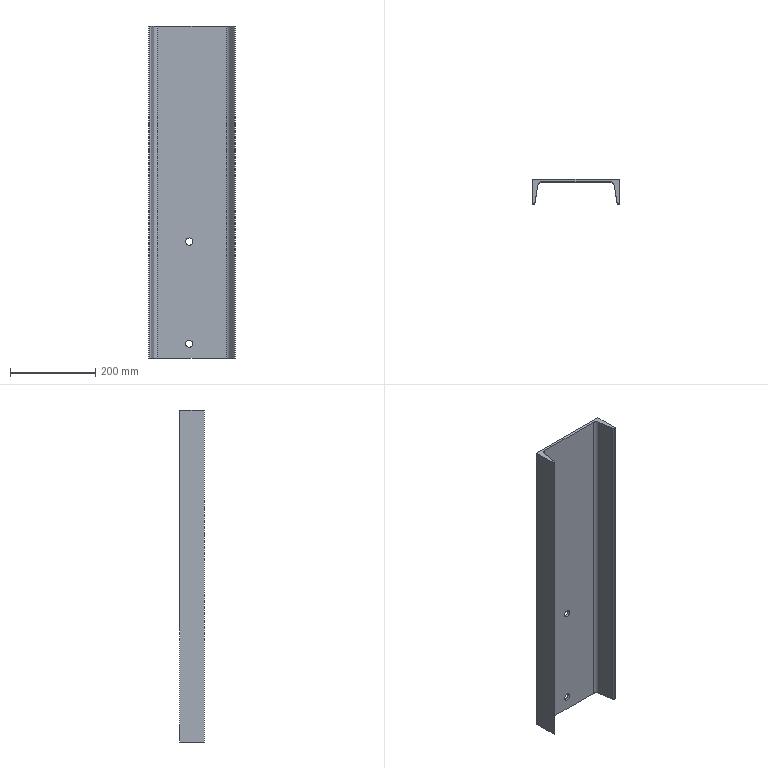Part | SolidWorks | features BaseBody 1 | 1 solid | 18 faces | box 203.2 x 57.4 x 780 mm | volume 1609191 mm3 | plane 10 | cylinder 8 | commonest cylinder face diameters 17 x4 6.6 x2 17.8 x2
STEP:
#1=CARTESIAN_POINT('',(61.02,28.984,265.));
#2=VERTEX_POINT('',#1);
#3=CARTESIAN_POINT('',(61.02,28.984,282.));
#4=VERTEX_POINT('',#3);
#5=CARTESIAN_POINT('',(61.02,28.984,273.5));
#6=DIRECTION('',(0.,1.,0.));
#7=DIRECTION('',(0.,0.,1.));
#8=AXIS2_PLACEMENT_3D('',#5,#6,#7);
#9=CIRCLE('',#8,8.5);
#10=EDGE_CURVE('',#2,#4,#9,.T.);
#11=ORIENTED_EDGE('',*,*,#10,.F.);
#12=CARTESIAN_POINT('',(61.02,34.584,265.));
#13=VERTEX_POINT('',#12);
#14=CARTESIAN_POINT('',(61.02,29.584,265.));
#15=DIRECTION('',(0.,1.,0.));
#16=VECTOR('',#15,1000.);
#17=LINE('',#14,#16);
#18=EDGE_CURVE('',#2,#13,#17,.T.);
#19=ORIENTED_EDGE('',*,*,#18,.T.);
#20=CARTESIAN_POINT('',(61.02,34.584,282.));
#21=VERTEX_POINT('',#20);
#22=CARTESIAN_POINT('',(61.02,34.584,273.5));
#23=DIRECTION('',(0.,-1.,0.));
#24=DIRECTION('',(0.,0.,1.));
#25=AXIS2_PLACEMENT_3D('',#22,#23,#24);
#26=CIRCLE('',#25,8.5);
#27=EDGE_CURVE('',#21,#13,#26,.T.);
#28=ORIENTED_EDGE('',*,*,#27,.F.);
#29=CARTESIAN_POINT('',(61.02,29.584,282.));
#30=DIRECTION('',(0.,1.,0.));
#31=VECTOR('',#30,1000.);
#32=LINE('',#29,#31);
#33=EDGE_CURVE('',#4,#21,#32,.T.);
#34=ORIENTED_EDGE('',*,*,#33,.F.);
#35=EDGE_LOOP('',(#11,#19,#28,#34));
#36=FACE_OUTER_BOUND('',#35,.T.);
#37=CARTESIAN_POINT('',(61.02,29.584,273.5));
#38=DIRECTION('',(0.,1.,0.));
#39=DIRECTION('',(0.,0.,1.));
#40=AXIS2_PLACEMENT_3D('',#37,#38,#39);
#41=CYLINDRICAL_SURFACE('',#40,8.5);
#42=ADVANCED_FACE('',(#36),#41,.F.);
#43=CARTESIAN_POINT('',(61.249,28.984,25.));
#44=VERTEX_POINT('',#43);
#45=CARTESIAN_POINT('',(61.249,28.984,42.));
#46=VERTEX_POINT('',#45);
#47=CARTESIAN_POINT('',(61.249,28.984,33.5));
#48=DIRECTION('',(0.,1.,0.));
#49=DIRECTION('',(0.,0.,1.));
#50=AXIS2_PLACEMENT_3D('',#47,#48,#49);
#51=CIRCLE('',#50,8.5);
#52=EDGE_CURVE('',#44,#46,#51,.T.);
#53=ORIENTED_EDGE('',*,*,#52,.F.);
#54=CARTESIAN_POINT('',(61.249,34.584,25.));
#55=VERTEX_POINT('',#54);
#56=CARTESIAN_POINT('',(61.249,29.584,25.));
#57=DIRECTION('',(0.,1.,0.));
#58=VECTOR('',#57,1000.);
#59=LINE('',#56,#58);
#60=EDGE_CURVE('',#44,#55,#59,.T.);
#61=ORIENTED_EDGE('',*,*,#60,.T.);
#62=CARTESIAN_POINT('',(61.249,34.584,42.));
#63=VERTEX_POINT('',#62);
#64=CARTESIAN_POINT('',(61.249,34.584,33.5));
#65=DIRECTION('',(0.,-1.,0.));
#66=DIRECTION('',(0.,0.,1.));
#67=AXIS2_PLACEMENT_3D('',#64,#65,#66);
#68=CIRCLE('',#67,8.5);
#69=EDGE_CURVE('',#63,#55,#68,.T.);
#70=ORIENTED_EDGE('',*,*,#69,.F.);
#71=CARTESIAN_POINT('',(61.249,29.584,42.));
#72=DIRECTION('',(0.,1.,0.));
#73=VECTOR('',#72,1000.);
#74=LINE('',#71,#73);
#75=EDGE_CURVE('',#46,#63,#74,.T.);
#76=ORIENTED_EDGE('',*,*,#75,.F.);
#77=EDGE_LOOP('',(#53,#61,#70,#76));
#78=FACE_OUTER_BOUND('',#77,.T.);
#79=CARTESIAN_POINT('',(61.249,29.584,33.5));
#80=DIRECTION('',(0.,1.,0.));
#81=DIRECTION('',(0.,0.,1.));
#82=AXIS2_PLACEMENT_3D('',#79,#80,#81);
#83=CYLINDRICAL_SURFACE('',#82,8.5);
#84=ADVANCED_FACE('',(#78),#83,.F.);
#85=ORIENTED_EDGE('',*,*,#27,.T.);
#86=CARTESIAN_POINT('',(61.02,34.584,273.5));
#87=DIRECTION('',(0.,-1.,0.));
#88=DIRECTION('',(0.,0.,1.));
#89=AXIS2_PLACEMENT_3D('',#86,#87,#88);
#90=CIRCLE('',#89,8.5);
#91=EDGE_CURVE('',#13,#21,#90,.T.);
#92=ORIENTED_EDGE('',*,*,#91,.T.);
#93=EDGE_LOOP('',(#85,#92));
#94=FACE_BOUND('',#93,.T.);
#95=ORIENTED_EDGE('',*,*,#69,.T.);
#96=CARTESIAN_POINT('',(61.249,34.584,33.5));
#97=DIRECTION('',(0.,-1.,0.));
#98=DIRECTION('',(0.,0.,1.));
#99=AXIS2_PLACEMENT_3D('',#96,#97,#98);
#100=CIRCLE('',#99,8.5);
#101=EDGE_CURVE('',#55,#63,#100,.T.);
#102=ORIENTED_EDGE('',*,*,#101,.T.);
#103=EDGE_LOOP('',(#95,#102));
#104=FACE_BOUND('',#103,.T.);
#105=CARTESIAN_POINT('',(169.22,34.584,0.));
#106=VERTEX_POINT('',#105);
#107=CARTESIAN_POINT('',(-33.98,34.584,0.));
#108=VERTEX_POINT('',#107);
#109=CARTESIAN_POINT('',(-33.98,34.584,0.));
#110=DIRECTION('',(-1.,0.,0.));
#111=VECTOR('',#110,1000.);
#112=LINE('',#109,#111);
#113=EDGE_CURVE('',#106,#108,#112,.T.);
#114=ORIENTED_EDGE('',*,*,#113,.T.);
#115=CARTESIAN_POINT('',(-33.98,34.584,780.));
#116=VERTEX_POINT('',#115);
#117=CARTESIAN_POINT('',(-33.98,34.584,0.));
#118=DIRECTION('',(0.,0.,1.));
#119=VECTOR('',#118,1000.);
#120=LINE('',#117,#119);
#121=EDGE_CURVE('',#108,#116,#120,.T.);
#122=ORIENTED_EDGE('',*,*,#121,.T.);
#123=CARTESIAN_POINT('',(169.22,34.584,780.));
#124=VERTEX_POINT('',#123);
#125=CARTESIAN_POINT('',(-33.98,34.584,780.));
#126=DIRECTION('',(1.,0.,0.));
#127=VECTOR('',#126,1000.);
#128=LINE('',#125,#127);
#129=EDGE_CURVE('',#116,#124,#128,.T.);
#130=ORIENTED_EDGE('',*,*,#129,.T.);
#131=CARTESIAN_POINT('',(169.22,34.584,0.));
#132=DIRECTION('',(0.,0.,-1.));
#133=VECTOR('',#132,1000.);
#134=LINE('',#131,#133);
#135=EDGE_CURVE('',#124,#106,#134,.T.);
#136=ORIENTED_EDGE('',*,*,#135,.T.);
#137=EDGE_LOOP('',(#114,#122,#130,#136));
#138=FACE_OUTER_BOUND('',#137,.T.);
#139=CARTESIAN_POINT('',(-33.98,34.584,0.));
#140=DIRECTION('',(0.,1.,0.));
#141=DIRECTION('',(0.,0.,1.));
#142=AXIS2_PLACEMENT_3D('',#139,#140,#141);
#143=PLANE('',#142);
#144=ADVANCED_FACE('',(#94,#104,#138),#143,.T.);
#145=ORIENTED_EDGE('',*,*,#18,.F.);
#146=CARTESIAN_POINT('',(61.02,28.984,273.5));
#147=DIRECTION('',(0.,1.,0.));
#148=DIRECTION('',(0.,0.,1.));
#149=AXIS2_PLACEMENT_3D('',#146,#147,#148);
#150=CIRCLE('',#149,8.5);
#151=EDGE_CURVE('',#4,#2,#150,.T.);
#152=ORIENTED_EDGE('',*,*,#151,.F.);
#153=ORIENTED_EDGE('',*,*,#33,.T.);
#154=ORIENTED_EDGE('',*,*,#91,.F.);
#155=EDGE_LOOP('',(#145,#152,#153,#154));
#156=FACE_OUTER_BOUND('',#155,.T.);
#157=CARTESIAN_POINT('',(61.02,29.584,273.5));
#158=DIRECTION('',(0.,1.,0.));
#159=DIRECTION('',(0.,0.,1.));
#160=AXIS2_PLACEMENT_3D('',#157,#158,#159);
#161=CYLINDRICAL_SURFACE('',#160,8.5);
#162=ADVANCED_FACE('',(#156),#161,.F.);
#163=ORIENTED_EDGE('',*,*,#60,.F.);
#164=CARTESIAN_POINT('',(61.249,28.984,33.5));
#165=DIRECTION('',(0.,1.,0.));
#166=DIRECTION('',(0.,0.,1.));
#167=AXIS2_PLACEMENT_3D('',#164,#165,#166);
#168=CIRCLE('',#167,8.5);
#169=EDGE_CURVE('',#46,#44,#168,.T.);
#170=ORIENTED_EDGE('',*,*,#169,.F.);
#171=ORIENTED_EDGE('',*,*,#75,.T.);
#172=ORIENTED_EDGE('',*,*,#101,.F.);
#173=EDGE_LOOP('',(#163,#170,#171,#172));
#174=FACE_OUTER_BOUND('',#173,.T.);
#175=CARTESIAN_POINT('',(61.249,29.584,33.5));
#176=DIRECTION('',(0.,1.,0.));
#177=DIRECTION('',(0.,0.,1.));
#178=AXIS2_PLACEMENT_3D('',#175,#176,#177);
#179=CYLINDRICAL_SURFACE('',#178,8.5);
#180=ADVANCED_FACE('',(#174),#179,.F.);
#181=CARTESIAN_POINT('',(-33.98,-22.816,0.));
#182=VERTEX_POINT('',#181);
#183=CARTESIAN_POINT('',(-33.98,-22.816,0.));
#184=DIRECTION('',(0.,-1.,0.));
#185=VECTOR('',#184,1000.);
#186=LINE('',#183,#185);
#187=EDGE_CURVE('',#108,#182,#186,.T.);
#188=ORIENTED_EDGE('',*,*,#187,.T.);
#189=CARTESIAN_POINT('',(-33.98,-22.816,780.));
#190=VERTEX_POINT('',#189);
#191=CARTESIAN_POINT('',(-33.98,-22.816,0.));
#192=DIRECTION('',(0.,0.,1.));
#193=VECTOR('',#192,1000.);
#194=LINE('',#191,#193);
#195=EDGE_CURVE('',#182,#190,#194,.T.);
#196=ORIENTED_EDGE('',*,*,#195,.T.);
#197=CARTESIAN_POINT('',(-33.98,-22.816,780.));
#198=DIRECTION('',(0.,1.,0.));
#199=VECTOR('',#198,1000.);
#200=LINE('',#197,#199);
#201=EDGE_CURVE('',#190,#116,#200,.T.);
#202=ORIENTED_EDGE('',*,*,#201,.T.);
#203=ORIENTED_EDGE('',*,*,#121,.F.);
#204=EDGE_LOOP('',(#188,#196,#202,#203));
#205=FACE_OUTER_BOUND('',#204,.T.);
#206=CARTESIAN_POINT('',(-33.98,-22.816,0.));
#207=DIRECTION('',(-1.,0.,0.));
#208=DIRECTION('',(0.,0.,1.));
#209=AXIS2_PLACEMENT_3D('',#206,#207,#208);
#210=PLANE('',#209);
#211=ADVANCED_FACE('',(#205),#210,.T.);
#212=CARTESIAN_POINT('',(167.576,-22.816,0.));
#213=VERTEX_POINT('',#212);
#214=CARTESIAN_POINT('',(169.22,-22.816,0.));
#215=VERTEX_POINT('',#214);
#216=CARTESIAN_POINT('',(169.22,-22.816,0.));
#217=DIRECTION('',(1.,0.,0.));
#218=VECTOR('',#217,1000.);
#219=LINE('',#216,#218);
#220=EDGE_CURVE('',#213,#215,#219,.T.);
#221=ORIENTED_EDGE('',*,*,#220,.F.);
#222=CARTESIAN_POINT('',(164.321,-20.06,0.));
#223=VERTEX_POINT('',#222);
#224=CARTESIAN_POINT('',(167.576,-19.516,0.));
#225=DIRECTION('',(0.,0.,1.));
#226=DIRECTION('',(1.,0.,0.));
#227=AXIS2_PLACEMENT_3D('',#224,#225,#226);
#228=CIRCLE('',#227,3.3);
#229=EDGE_CURVE('',#223,#213,#228,.T.);
#230=ORIENTED_EDGE('',*,*,#229,.F.);
#231=CARTESIAN_POINT('',(157.358,21.553,0.));
#232=VERTEX_POINT('',#231);
#233=CARTESIAN_POINT('',(157.358,21.553,0.));
#234=DIRECTION('',(0.165,-0.9863,0.));
#235=VECTOR('',#234,1000.);
#236=LINE('',#233,#235);
#237=EDGE_CURVE('',#232,#223,#236,.T.);
#238=ORIENTED_EDGE('',*,*,#237,.F.);
#239=CARTESIAN_POINT('',(148.58,28.984,0.));
#240=VERTEX_POINT('',#239);
#241=CARTESIAN_POINT('',(148.58,20.084,0.));
#242=DIRECTION('',(0.,0.,-1.));
#243=DIRECTION('',(1.,0.,0.));
#244=AXIS2_PLACEMENT_3D('',#241,#242,#243);
#245=CIRCLE('',#244,8.9);
#246=EDGE_CURVE('',#240,#232,#245,.T.);
#247=ORIENTED_EDGE('',*,*,#246,.F.);
#248=CARTESIAN_POINT('',(-13.34,28.984,0.));
#249=VERTEX_POINT('',#248);
#250=CARTESIAN_POINT('',(67.62,28.984,0.));
#251=DIRECTION('',(1.,0.,0.));
#252=VECTOR('',#251,1000.);
#253=LINE('',#250,#252);
#254=EDGE_CURVE('',#249,#240,#253,.T.);
#255=ORIENTED_EDGE('',*,*,#254,.F.);
#256=CARTESIAN_POINT('',(-22.118,21.553,0.));
#257=VERTEX_POINT('',#256);
#258=CARTESIAN_POINT('',(-13.34,20.084,0.));
#259=DIRECTION('',(0.,0.,-1.));
#260=DIRECTION('',(1.,0.,0.));
#261=AXIS2_PLACEMENT_3D('',#258,#259,#260);
#262=CIRCLE('',#261,8.9);
#263=EDGE_CURVE('',#257,#249,#262,.T.);
#264=ORIENTED_EDGE('',*,*,#263,.F.);
#265=CARTESIAN_POINT('',(-29.082,-20.06,0.));
#266=VERTEX_POINT('',#265);
#267=CARTESIAN_POINT('',(-29.082,-20.06,0.));
#268=DIRECTION('',(0.165,0.9863,0.));
#269=VECTOR('',#268,1000.);
#270=LINE('',#267,#269);
#271=EDGE_CURVE('',#266,#257,#270,.T.);
#272=ORIENTED_EDGE('',*,*,#271,.F.);
#273=CARTESIAN_POINT('',(-32.337,-22.816,0.));
#274=VERTEX_POINT('',#273);
#275=CARTESIAN_POINT('',(-32.337,-19.516,0.));
#276=DIRECTION('',(0.,0.,1.));
#277=DIRECTION('',(1.,0.,0.));
#278=AXIS2_PLACEMENT_3D('',#275,#276,#277);
#279=CIRCLE('',#278,3.3);
#280=EDGE_CURVE('',#274,#266,#279,.T.);
#281=ORIENTED_EDGE('',*,*,#280,.F.);
#282=CARTESIAN_POINT('',(67.62,-22.816,0.));
#283=DIRECTION('',(1.,0.,0.));
#284=VECTOR('',#283,1000.);
#285=LINE('',#282,#284);
#286=EDGE_CURVE('',#182,#274,#285,.T.);
#287=ORIENTED_EDGE('',*,*,#286,.F.);
#288=ORIENTED_EDGE('',*,*,#187,.F.);
#289=ORIENTED_EDGE('',*,*,#113,.F.);
#290=CARTESIAN_POINT('',(169.22,21.33,0.));
#291=DIRECTION('',(0.,1.,0.));
#292=VECTOR('',#291,1000.);
#293=LINE('',#290,#292);
#294=EDGE_CURVE('',#215,#106,#293,.T.);
#295=ORIENTED_EDGE('',*,*,#294,.F.);
#296=EDGE_LOOP('',(#221,#230,#238,#247,#255,#264,#272,#281,#287,#288,#289,#295));
#297=FACE_OUTER_BOUND('',#296,.T.);
#298=CARTESIAN_POINT('',(67.62,21.33,0.));
#299=DIRECTION('',(0.,0.,1.));
#300=DIRECTION('',(1.,0.,0.));
#301=AXIS2_PLACEMENT_3D('',#298,#299,#300);
#302=PLANE('',#301);
#303=ADVANCED_FACE('',(#297),#302,.F.);
#304=ORIENTED_EDGE('',*,*,#294,.T.);
#305=ORIENTED_EDGE('',*,*,#135,.F.);
#306=CARTESIAN_POINT('',(169.22,-22.816,780.));
#307=VERTEX_POINT('',#306);
#308=CARTESIAN_POINT('',(169.22,34.584,780.));
#309=DIRECTION('',(0.,-1.,0.));
#310=VECTOR('',#309,1000.);
#311=LINE('',#308,#310);
#312=EDGE_CURVE('',#124,#307,#311,.T.);
#313=ORIENTED_EDGE('',*,*,#312,.T.);
#314=CARTESIAN_POINT('',(169.22,-22.816,0.));
#315=DIRECTION('',(0.,0.,-1.));
#316=VECTOR('',#315,1000.);
#317=LINE('',#314,#316);
#318=EDGE_CURVE('',#307,#215,#317,.T.);
#319=ORIENTED_EDGE('',*,*,#318,.T.);
#320=EDGE_LOOP('',(#304,#305,#313,#319));
#321=FACE_OUTER_BOUND('',#320,.T.);
#322=CARTESIAN_POINT('',(169.22,34.584,0.));
#323=DIRECTION('',(1.,0.,0.));
#324=DIRECTION('',(0.,0.,-1.));
#325=AXIS2_PLACEMENT_3D('',#322,#323,#324);
#326=PLANE('',#325);
#327=ADVANCED_FACE('',(#321),#326,.T.);
#328=CARTESIAN_POINT('',(157.358,21.553,780.));
#329=VERTEX_POINT('',#328);
#330=CARTESIAN_POINT('',(164.321,-20.06,780.));
#331=VERTEX_POINT('',#330);
#332=CARTESIAN_POINT('',(157.358,21.553,780.));
#333=DIRECTION('',(0.165,-0.9863,0.));
#334=VECTOR('',#333,1000.);
#335=LINE('',#332,#334);
#336=EDGE_CURVE('',#329,#331,#335,.T.);
#337=ORIENTED_EDGE('',*,*,#336,.T.);
#338=CARTESIAN_POINT('',(167.576,-22.816,780.));
#339=VERTEX_POINT('',#338);
#340=CARTESIAN_POINT('',(167.576,-19.516,780.));
#341=DIRECTION('',(0.,0.,1.));
#342=DIRECTION('',(1.,0.,0.));
#343=AXIS2_PLACEMENT_3D('',#340,#341,#342);
#344=CIRCLE('',#343,3.3);
#345=EDGE_CURVE('',#331,#339,#344,.T.);
#346=ORIENTED_EDGE('',*,*,#345,.T.);
#347=CARTESIAN_POINT('',(67.62,-22.816,780.));
#348=DIRECTION('',(1.,0.,0.));
#349=VECTOR('',#348,1000.);
#350=LINE('',#347,#349);
#351=EDGE_CURVE('',#339,#307,#350,.T.);
#352=ORIENTED_EDGE('',*,*,#351,.T.);
#353=ORIENTED_EDGE('',*,*,#312,.F.);
#354=ORIENTED_EDGE('',*,*,#129,.F.);
#355=ORIENTED_EDGE('',*,*,#201,.F.);
#356=CARTESIAN_POINT('',(-32.337,-22.816,780.));
#357=VERTEX_POINT('',#356);
#358=CARTESIAN_POINT('',(67.62,-22.816,780.));
#359=DIRECTION('',(1.,0.,0.));
#360=VECTOR('',#359,1000.);
#361=LINE('',#358,#360);
#362=EDGE_CURVE('',#190,#357,#361,.T.);
#363=ORIENTED_EDGE('',*,*,#362,.T.);
#364=CARTESIAN_POINT('',(-29.082,-20.06,780.));
#365=VERTEX_POINT('',#364);
#366=CARTESIAN_POINT('',(-32.337,-19.516,780.));
#367=DIRECTION('',(0.,0.,1.));
#368=DIRECTION('',(1.,0.,0.));
#369=AXIS2_PLACEMENT_3D('',#366,#367,#368);
#370=CIRCLE('',#369,3.3);
#371=EDGE_CURVE('',#357,#365,#370,.T.);
#372=ORIENTED_EDGE('',*,*,#371,.T.);
#373=CARTESIAN_POINT('',(-22.118,21.553,780.));
#374=VERTEX_POINT('',#373);
#375=CARTESIAN_POINT('',(-29.082,-20.06,780.));
#376=DIRECTION('',(0.165,0.9863,0.));
#377=VECTOR('',#376,1000.);
#378=LINE('',#375,#377);
#379=EDGE_CURVE('',#365,#374,#378,.T.);
#380=ORIENTED_EDGE('',*,*,#379,.T.);
#381=CARTESIAN_POINT('',(-13.34,28.984,780.));
#382=VERTEX_POINT('',#381);
#383=CARTESIAN_POINT('',(-13.34,20.084,780.));
#384=DIRECTION('',(0.,0.,-1.));
#385=DIRECTION('',(1.,0.,0.));
#386=AXIS2_PLACEMENT_3D('',#383,#384,#385);
#387=CIRCLE('',#386,8.9);
#388=EDGE_CURVE('',#374,#382,#387,.T.);
#389=ORIENTED_EDGE('',*,*,#388,.T.);
#390=CARTESIAN_POINT('',(148.58,28.984,780.));
#391=VERTEX_POINT('',#390);
#392=CARTESIAN_POINT('',(67.62,28.984,780.));
#393=DIRECTION('',(1.,0.,0.));
#394=VECTOR('',#393,1000.);
#395=LINE('',#392,#394);
#396=EDGE_CURVE('',#382,#391,#395,.T.);
#397=ORIENTED_EDGE('',*,*,#396,.T.);
#398=CARTESIAN_POINT('',(148.58,20.084,780.));
#399=DIRECTION('',(0.,0.,-1.));
#400=DIRECTION('',(1.,0.,0.));
#401=AXIS2_PLACEMENT_3D('',#398,#399,#400);
#402=CIRCLE('',#401,8.9);
#403=EDGE_CURVE('',#391,#329,#402,.T.);
#404=ORIENTED_EDGE('',*,*,#403,.T.);
#405=EDGE_LOOP('',(#337,#346,#352,#353,#354,#355,#363,#372,#380,#389,#397,#404));
#406=FACE_OUTER_BOUND('',#405,.T.);
#407=CARTESIAN_POINT('',(67.62,21.33,780.));
#408=DIRECTION('',(0.,0.,1.));
#409=DIRECTION('',(1.,0.,0.));
#410=AXIS2_PLACEMENT_3D('',#407,#408,#409);
#411=PLANE('',#410);
#412=ADVANCED_FACE('',(#406),#411,.T.);
#413=ORIENTED_EDGE('',*,*,#151,.T.);
#414=ORIENTED_EDGE('',*,*,#10,.T.);
#415=EDGE_LOOP('',(#413,#414));
#416=FACE_BOUND('',#415,.T.);
#417=ORIENTED_EDGE('',*,*,#169,.T.);
#418=ORIENTED_EDGE('',*,*,#52,.T.);
#419=EDGE_LOOP('',(#417,#418));
#420=FACE_BOUND('',#419,.T.);
#421=ORIENTED_EDGE('',*,*,#254,.T.);
#422=CARTESIAN_POINT('',(148.58,28.984,0.));
#423=DIRECTION('',(0.,0.,1.));
#424=VECTOR('',#423,1000.);
#425=LINE('',#422,#424);
#426=EDGE_CURVE('',#240,#391,#425,.T.);
#427=ORIENTED_EDGE('',*,*,#426,.T.);
#428=ORIENTED_EDGE('',*,*,#396,.F.);
#429=CARTESIAN_POINT('',(-13.34,28.984,0.));
#430=DIRECTION('',(0.,0.,-1.));
#431=VECTOR('',#430,1000.);
#432=LINE('',#429,#431);
#433=EDGE_CURVE('',#382,#249,#432,.T.);
#434=ORIENTED_EDGE('',*,*,#433,.T.);
#435=EDGE_LOOP('',(#421,#427,#428,#434));
#436=FACE_OUTER_BOUND('',#435,.T.);
#437=CARTESIAN_POINT('',(148.58,28.984,0.));
#438=DIRECTION('',(0.,-1.,0.));
#439=DIRECTION('',(1.,0.,0.));
#440=AXIS2_PLACEMENT_3D('',#437,#438,#439);
#441=PLANE('',#440);
#442=ADVANCED_FACE('',(#416,#420,#436),#441,.T.);
#443=ORIENTED_EDGE('',*,*,#286,.T.);
#444=CARTESIAN_POINT('',(-32.337,-22.816,0.));
#445=DIRECTION('',(0.,0.,1.));
#446=VECTOR('',#445,1000.);
#447=LINE('',#444,#446);
#448=EDGE_CURVE('',#274,#357,#447,.T.);
#449=ORIENTED_EDGE('',*,*,#448,.T.);
#450=ORIENTED_EDGE('',*,*,#362,.F.);
#451=ORIENTED_EDGE('',*,*,#195,.F.);
#452=EDGE_LOOP('',(#443,#449,#450,#451));
#453=FACE_OUTER_BOUND('',#452,.T.);
#454=CARTESIAN_POINT('',(-32.337,-22.816,0.));
#455=DIRECTION('',(0.,-1.,0.));
#456=DIRECTION('',(1.,0.,0.));
#457=AXIS2_PLACEMENT_3D('',#454,#455,#456);
#458=PLANE('',#457);
#459=ADVANCED_FACE('',(#453),#458,.T.);
#460=ORIENTED_EDGE('',*,*,#229,.T.);
#461=CARTESIAN_POINT('',(167.576,-22.816,0.));
#462=DIRECTION('',(0.,0.,1.));
#463=VECTOR('',#462,1000.);
#464=LINE('',#461,#463);
#465=EDGE_CURVE('',#213,#339,#464,.T.);
#466=ORIENTED_EDGE('',*,*,#465,.T.);
#467=ORIENTED_EDGE('',*,*,#345,.F.);
#468=CARTESIAN_POINT('',(164.321,-20.06,0.));
#469=DIRECTION('',(0.,0.,-1.));
#470=VECTOR('',#469,1000.);
#471=LINE('',#468,#470);
#472=EDGE_CURVE('',#331,#223,#471,.T.);
#473=ORIENTED_EDGE('',*,*,#472,.T.);
#474=EDGE_LOOP('',(#460,#466,#467,#473));
#475=FACE_OUTER_BOUND('',#474,.T.);
#476=CARTESIAN_POINT('',(167.576,-19.516,0.));
#477=DIRECTION('',(0.,0.,1.));
#478=DIRECTION('',(1.,0.,0.));
#479=AXIS2_PLACEMENT_3D('',#476,#477,#478);
#480=CYLINDRICAL_SURFACE('',#479,3.3);
#481=ADVANCED_FACE('',(#475),#480,.T.);
#482=ORIENTED_EDGE('',*,*,#237,.T.);
#483=ORIENTED_EDGE('',*,*,#472,.F.);
#484=ORIENTED_EDGE('',*,*,#336,.F.);
#485=CARTESIAN_POINT('',(157.358,21.553,0.));
#486=DIRECTION('',(0.,0.,-1.));
#487=VECTOR('',#486,1000.);
#488=LINE('',#485,#487);
#489=EDGE_CURVE('',#329,#232,#488,.T.);
#490=ORIENTED_EDGE('',*,*,#489,.T.);
#491=EDGE_LOOP('',(#482,#483,#484,#490));
#492=FACE_OUTER_BOUND('',#491,.T.);
#493=CARTESIAN_POINT('',(164.321,-20.06,0.));
#494=DIRECTION('',(-0.9863,-0.165,0.));
#495=DIRECTION('',(0.165,-0.9863,0.));
#496=AXIS2_PLACEMENT_3D('',#493,#494,#495);
#497=PLANE('',#496);
#498=ADVANCED_FACE('',(#492),#497,.T.);
#499=ORIENTED_EDGE('',*,*,#426,.F.);
#500=ORIENTED_EDGE('',*,*,#246,.T.);
#501=ORIENTED_EDGE('',*,*,#489,.F.);
#502=ORIENTED_EDGE('',*,*,#403,.F.);
#503=EDGE_LOOP('',(#499,#500,#501,#502));
#504=FACE_OUTER_BOUND('',#503,.T.);
#505=CARTESIAN_POINT('',(148.58,20.084,0.));
#506=DIRECTION('',(0.,0.,1.));
#507=DIRECTION('',(1.,0.,0.));
#508=AXIS2_PLACEMENT_3D('',#505,#506,#507);
#509=CYLINDRICAL_SURFACE('',#508,8.9);
#510=ADVANCED_FACE('',(#504),#509,.F.);
#511=CARTESIAN_POINT('',(-22.118,21.553,0.));
#512=DIRECTION('',(0.,0.,1.));
#513=VECTOR('',#512,1000.);
#514=LINE('',#511,#513);
#515=EDGE_CURVE('',#257,#374,#514,.T.);
#516=ORIENTED_EDGE('',*,*,#515,.F.);
#517=ORIENTED_EDGE('',*,*,#263,.T.);
#518=ORIENTED_EDGE('',*,*,#433,.F.);
#519=ORIENTED_EDGE('',*,*,#388,.F.);
#520=EDGE_LOOP('',(#516,#517,#518,#519));
#521=FACE_OUTER_BOUND('',#520,.T.);
#522=CARTESIAN_POINT('',(-13.34,20.084,0.));
#523=DIRECTION('',(0.,0.,1.));
#524=DIRECTION('',(1.,0.,0.));
#525=AXIS2_PLACEMENT_3D('',#522,#523,#524);
#526=CYLINDRICAL_SURFACE('',#525,8.9);
#527=ADVANCED_FACE('',(#521),#526,.F.);
#528=ORIENTED_EDGE('',*,*,#271,.T.);
#529=ORIENTED_EDGE('',*,*,#515,.T.);
#530=ORIENTED_EDGE('',*,*,#379,.F.);
#531=CARTESIAN_POINT('',(-29.082,-20.06,0.));
#532=DIRECTION('',(0.,0.,-1.));
#533=VECTOR('',#532,1000.);
#534=LINE('',#531,#533);
#535=EDGE_CURVE('',#365,#266,#534,.T.);
#536=ORIENTED_EDGE('',*,*,#535,.T.);
#537=EDGE_LOOP('',(#528,#529,#530,#536));
#538=FACE_OUTER_BOUND('',#537,.T.);
#539=CARTESIAN_POINT('',(-22.118,21.553,0.));
#540=DIRECTION('',(0.9863,-0.165,0.));
#541=DIRECTION('',(0.165,0.9863,0.));
#542=AXIS2_PLACEMENT_3D('',#539,#540,#541);
#543=PLANE('',#542);
#544=ADVANCED_FACE('',(#538),#543,.T.);
#545=ORIENTED_EDGE('',*,*,#280,.T.);
#546=ORIENTED_EDGE('',*,*,#535,.F.);
#547=ORIENTED_EDGE('',*,*,#371,.F.);
#548=ORIENTED_EDGE('',*,*,#448,.F.);
#549=EDGE_LOOP('',(#545,#546,#547,#548));
#550=FACE_OUTER_BOUND('',#549,.T.);
#551=CARTESIAN_POINT('',(-32.337,-19.516,0.));
#552=DIRECTION('',(0.,0.,1.));
#553=DIRECTION('',(1.,0.,0.));
#554=AXIS2_PLACEMENT_3D('',#551,#552,#553);
#555=CYLINDRICAL_SURFACE('',#554,3.3);
#556=ADVANCED_FACE('',(#550),#555,.T.);
#557=ORIENTED_EDGE('',*,*,#220,.T.);
#558=ORIENTED_EDGE('',*,*,#318,.F.);
#559=ORIENTED_EDGE('',*,*,#351,.F.);
#560=ORIENTED_EDGE('',*,*,#465,.F.);
#561=EDGE_LOOP('',(#557,#558,#559,#560));
#562=FACE_OUTER_BOUND('',#561,.T.);
#563=CARTESIAN_POINT('',(169.22,-22.816,0.));
#564=DIRECTION('',(0.,-1.,0.));
#565=DIRECTION('',(0.,0.,-1.));
#566=AXIS2_PLACEMENT_3D('',#563,#564,#565);
#567=PLANE('',#566);
#568=ADVANCED_FACE('',(#562),#567,.T.);
#569=CLOSED_SHELL('',(#42,#84,#144,#162,#180,#211,#303,#327,#412,#442,#459,#481,#498,#510,#527,#544,#556,#568));
#570=MANIFOLD_SOLID_BREP('',#569);
#571=CARTESIAN_POINT('',(0.,0.,0.));
#572=DIRECTION('',(0.,0.,1.));
#573=DIRECTION('',(1.,0.,0.));
#574=AXIS2_PLACEMENT_3D('',#571,#572,#573);
#575=(LENGTH_UNIT()NAMED_UNIT(*)SI_UNIT(.MILLI.,.METRE.));
#576=UNCERTAINTY_MEASURE_WITH_UNIT(LENGTH_MEASURE(0.00001),#575,'','');
#577=(NAMED_UNIT(*)PLANE_ANGLE_UNIT()SI_UNIT($,.RADIAN.));
#578=(NAMED_UNIT(*)SI_UNIT($,.STERADIAN.)SOLID_ANGLE_UNIT());
#579=(GEOMETRIC_REPRESENTATION_CONTEXT(3)GLOBAL_UNCERTAINTY_ASSIGNED_CONTEXT((#576))GLOBAL_UNIT_ASSIGNED_CONTEXT((#575,#577,#578))REPRESENTATION_CONTEXT('',''));
#580=ADVANCED_BREP_SHAPE_REPRESENTATION('',(#570,#574),#579);